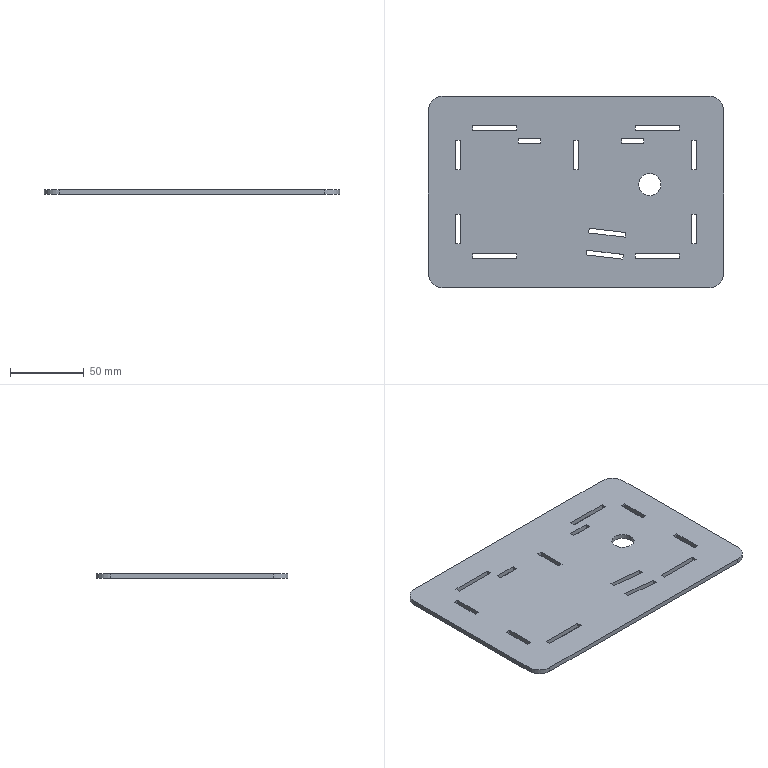Part | SolidWorks | features FlatPattern 1, SMBaseFlange 1, SheetMetal 1 | 1 solid | 64 faces | box 200 x 130 x 3.2 mm | volume 79288 mm3 | plane 58 | cylinder 6 | commonest cylinder face diameters 20 x4 15 x2